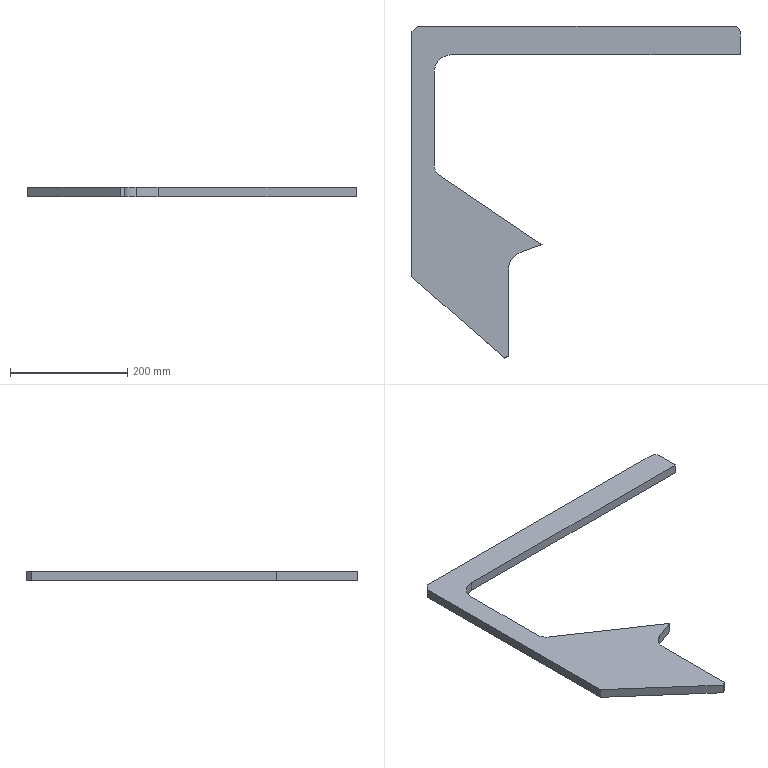Part | SolidWorks | features Extrusion 1 | 1 solid | 17 faces | box 560 x 566.399 x 16 mm | volume 1167723 mm3 | plane 13 | cylinder 4 | commonest cylinder face diameters 60 x2 20 x1 40 x1
STEP:
#1=CARTESIAN_POINT('',(560.,563.,0.));
#2=VERTEX_POINT('',#1);
#3=CARTESIAN_POINT('',(550.,573.,0.));
#4=VERTEX_POINT('',#3);
#5=CARTESIAN_POINT('',(550.,563.,0.));
#6=DIRECTION('',(0.,0.,1.));
#7=DIRECTION('',(1.,0.,0.));
#8=AXIS2_PLACEMENT_3D('',#5,#6,#7);
#9=CIRCLE('',#8,10.);
#10=EDGE_CURVE('',#2,#4,#9,.T.);
#11=ORIENTED_EDGE('',*,*,#10,.T.);
#12=CARTESIAN_POINT('',(550.,573.,16.));
#13=VERTEX_POINT('',#12);
#14=CARTESIAN_POINT('',(550.,573.,16.));
#15=DIRECTION('',(0.,0.,-1.));
#16=VECTOR('',#15,1000.);
#17=LINE('',#14,#16);
#18=EDGE_CURVE('',#13,#4,#17,.T.);
#19=ORIENTED_EDGE('',*,*,#18,.F.);
#20=CARTESIAN_POINT('',(560.,563.,16.));
#21=VERTEX_POINT('',#20);
#22=CARTESIAN_POINT('',(550.,563.,16.));
#23=DIRECTION('',(0.,0.,1.));
#24=DIRECTION('',(1.,0.,0.));
#25=AXIS2_PLACEMENT_3D('',#22,#23,#24);
#26=CIRCLE('',#25,10.);
#27=EDGE_CURVE('',#21,#13,#26,.T.);
#28=ORIENTED_EDGE('',*,*,#27,.F.);
#29=CARTESIAN_POINT('',(560.,563.,16.));
#30=DIRECTION('',(0.,0.,-1.));
#31=VECTOR('',#30,1000.);
#32=LINE('',#29,#31);
#33=EDGE_CURVE('',#21,#2,#32,.T.);
#34=ORIENTED_EDGE('',*,*,#33,.T.);
#35=EDGE_LOOP('',(#11,#19,#28,#34));
#36=FACE_OUTER_BOUND('',#35,.T.);
#37=CARTESIAN_POINT('',(550.,563.,16.));
#38=DIRECTION('',(0.,0.,-1.));
#39=DIRECTION('',(-1.,0.,0.));
#40=AXIS2_PLACEMENT_3D('',#37,#38,#39);
#41=CYLINDRICAL_SURFACE('',#40,10.);
#42=ADVANCED_FACE('',(#36),#41,.T.);
#43=CARTESIAN_POINT('',(10.,573.,0.));
#44=VERTEX_POINT('',#43);
#45=CARTESIAN_POINT('',(10.,573.,0.));
#46=DIRECTION('',(-1.,0.,0.));
#47=VECTOR('',#46,1000.);
#48=LINE('',#45,#47);
#49=EDGE_CURVE('',#4,#44,#48,.T.);
#50=ORIENTED_EDGE('',*,*,#49,.T.);
#51=CARTESIAN_POINT('',(10.,573.,16.));
#52=VERTEX_POINT('',#51);
#53=CARTESIAN_POINT('',(10.,573.,16.));
#54=DIRECTION('',(0.,0.,-1.));
#55=VECTOR('',#54,1000.);
#56=LINE('',#53,#55);
#57=EDGE_CURVE('',#52,#44,#56,.T.);
#58=ORIENTED_EDGE('',*,*,#57,.F.);
#59=CARTESIAN_POINT('',(10.,573.,16.));
#60=DIRECTION('',(-1.,0.,0.));
#61=VECTOR('',#60,1000.);
#62=LINE('',#59,#61);
#63=EDGE_CURVE('',#13,#52,#62,.T.);
#64=ORIENTED_EDGE('',*,*,#63,.F.);
#65=ORIENTED_EDGE('',*,*,#18,.T.);
#66=EDGE_LOOP('',(#50,#58,#64,#65));
#67=FACE_OUTER_BOUND('',#66,.T.);
#68=CARTESIAN_POINT('',(10.,573.,16.));
#69=DIRECTION('',(0.,-1.,0.));
#70=DIRECTION('',(0.,0.,-1.));
#71=AXIS2_PLACEMENT_3D('',#68,#69,#70);
#72=PLANE('',#71);
#73=ADVANCED_FACE('',(#67),#72,.F.);
#74=CARTESIAN_POINT('',(0.,563.,0.));
#75=VERTEX_POINT('',#74);
#76=CARTESIAN_POINT('',(0.,563.,0.));
#77=DIRECTION('',(-0.7071,-0.7071,0.));
#78=VECTOR('',#77,1000.);
#79=LINE('',#76,#78);
#80=EDGE_CURVE('',#44,#75,#79,.T.);
#81=ORIENTED_EDGE('',*,*,#80,.T.);
#82=CARTESIAN_POINT('',(0.,563.,16.));
#83=VERTEX_POINT('',#82);
#84=CARTESIAN_POINT('',(0.,563.,16.));
#85=DIRECTION('',(0.,0.,-1.));
#86=VECTOR('',#85,1000.);
#87=LINE('',#84,#86);
#88=EDGE_CURVE('',#83,#75,#87,.T.);
#89=ORIENTED_EDGE('',*,*,#88,.F.);
#90=CARTESIAN_POINT('',(0.,563.,16.));
#91=DIRECTION('',(-0.7071,-0.7071,0.));
#92=VECTOR('',#91,1000.);
#93=LINE('',#90,#92);
#94=EDGE_CURVE('',#52,#83,#93,.T.);
#95=ORIENTED_EDGE('',*,*,#94,.F.);
#96=ORIENTED_EDGE('',*,*,#57,.T.);
#97=EDGE_LOOP('',(#81,#89,#95,#96));
#98=FACE_OUTER_BOUND('',#97,.T.);
#99=CARTESIAN_POINT('',(0.,563.,16.));
#100=DIRECTION('',(0.7071,-0.7071,0.));
#101=DIRECTION('',(0.7071,0.7071,0.));
#102=AXIS2_PLACEMENT_3D('',#99,#100,#101);
#103=PLANE('',#102);
#104=ADVANCED_FACE('',(#98),#103,.F.);
#105=CARTESIAN_POINT('',(0.,145.,0.));
#106=VERTEX_POINT('',#105);
#107=CARTESIAN_POINT('',(0.,145.,0.));
#108=DIRECTION('',(0.,-1.,0.));
#109=VECTOR('',#108,1000.);
#110=LINE('',#107,#109);
#111=EDGE_CURVE('',#75,#106,#110,.T.);
#112=ORIENTED_EDGE('',*,*,#111,.T.);
#113=CARTESIAN_POINT('',(0.,145.,16.));
#114=VERTEX_POINT('',#113);
#115=CARTESIAN_POINT('',(0.,145.,16.));
#116=DIRECTION('',(0.,0.,-1.));
#117=VECTOR('',#116,1000.);
#118=LINE('',#115,#117);
#119=EDGE_CURVE('',#114,#106,#118,.T.);
#120=ORIENTED_EDGE('',*,*,#119,.F.);
#121=CARTESIAN_POINT('',(0.,145.,16.));
#122=DIRECTION('',(0.,-1.,0.));
#123=VECTOR('',#122,1000.);
#124=LINE('',#121,#123);
#125=EDGE_CURVE('',#83,#114,#124,.T.);
#126=ORIENTED_EDGE('',*,*,#125,.F.);
#127=ORIENTED_EDGE('',*,*,#88,.T.);
#128=EDGE_LOOP('',(#112,#120,#126,#127));
#129=FACE_OUTER_BOUND('',#128,.T.);
#130=CARTESIAN_POINT('',(0.,145.,16.));
#131=DIRECTION('',(1.,0.,0.));
#132=DIRECTION('',(0.,0.,-1.));
#133=AXIS2_PLACEMENT_3D('',#130,#131,#132);
#134=PLANE('',#133);
#135=ADVANCED_FACE('',(#129),#134,.F.);
#136=CARTESIAN_POINT('',(157.488,6.601,0.));
#137=VERTEX_POINT('',#136);
#138=CARTESIAN_POINT('',(157.488,6.601,0.));
#139=DIRECTION('',(0.7512,-0.6601,0.));
#140=VECTOR('',#139,1000.);
#141=LINE('',#138,#140);
#142=EDGE_CURVE('',#106,#137,#141,.T.);
#143=ORIENTED_EDGE('',*,*,#142,.T.);
#144=CARTESIAN_POINT('',(157.488,6.601,16.));
#145=VERTEX_POINT('',#144);
#146=CARTESIAN_POINT('',(157.488,6.601,16.));
#147=DIRECTION('',(0.,0.,-1.));
#148=VECTOR('',#147,1000.);
#149=LINE('',#146,#148);
#150=EDGE_CURVE('',#145,#137,#149,.T.);
#151=ORIENTED_EDGE('',*,*,#150,.F.);
#152=CARTESIAN_POINT('',(157.488,6.601,16.));
#153=DIRECTION('',(0.7512,-0.6601,0.));
#154=VECTOR('',#153,1000.);
#155=LINE('',#152,#154);
#156=EDGE_CURVE('',#114,#145,#155,.T.);
#157=ORIENTED_EDGE('',*,*,#156,.F.);
#158=ORIENTED_EDGE('',*,*,#119,.T.);
#159=EDGE_LOOP('',(#143,#151,#157,#158));
#160=FACE_OUTER_BOUND('',#159,.T.);
#161=CARTESIAN_POINT('',(157.488,6.601,16.));
#162=DIRECTION('',(0.6601,0.7512,0.));
#163=DIRECTION('',(-0.7512,0.6601,0.));
#164=AXIS2_PLACEMENT_3D('',#161,#162,#163);
#165=PLANE('',#164);
#166=ADVANCED_FACE('',(#160),#165,.F.);
#167=CARTESIAN_POINT('',(165.,10.,0.));
#168=VERTEX_POINT('',#167);
#169=CARTESIAN_POINT('',(165.,10.,0.));
#170=DIRECTION('',(0.9111,0.4122,0.));
#171=VECTOR('',#170,1000.);
#172=LINE('',#169,#171);
#173=EDGE_CURVE('',#137,#168,#172,.T.);
#174=ORIENTED_EDGE('',*,*,#173,.T.);
#175=CARTESIAN_POINT('',(165.,10.,16.));
#176=VERTEX_POINT('',#175);
#177=CARTESIAN_POINT('',(165.,10.,16.));
#178=DIRECTION('',(0.,0.,-1.));
#179=VECTOR('',#178,1000.);
#180=LINE('',#177,#179);
#181=EDGE_CURVE('',#176,#168,#180,.T.);
#182=ORIENTED_EDGE('',*,*,#181,.F.);
#183=CARTESIAN_POINT('',(165.,10.,16.));
#184=DIRECTION('',(0.9111,0.4122,0.));
#185=VECTOR('',#184,1000.);
#186=LINE('',#183,#185);
#187=EDGE_CURVE('',#145,#176,#186,.T.);
#188=ORIENTED_EDGE('',*,*,#187,.F.);
#189=ORIENTED_EDGE('',*,*,#150,.T.);
#190=EDGE_LOOP('',(#174,#182,#188,#189));
#191=FACE_OUTER_BOUND('',#190,.T.);
#192=CARTESIAN_POINT('',(165.,10.,16.));
#193=DIRECTION('',(-0.4122,0.9111,0.));
#194=DIRECTION('',(-0.9111,-0.4122,0.));
#195=AXIS2_PLACEMENT_3D('',#192,#193,#194);
#196=PLANE('',#195);
#197=ADVANCED_FACE('',(#191),#196,.F.);
#198=CARTESIAN_POINT('',(165.,158.408,0.));
#199=VERTEX_POINT('',#198);
#200=CARTESIAN_POINT('',(165.,158.408,0.));
#201=DIRECTION('',(0.,1.,0.));
#202=VECTOR('',#201,1000.);
#203=LINE('',#200,#202);
#204=EDGE_CURVE('',#168,#199,#203,.T.);
#205=ORIENTED_EDGE('',*,*,#204,.T.);
#206=CARTESIAN_POINT('',(165.,158.408,16.));
#207=VERTEX_POINT('',#206);
#208=CARTESIAN_POINT('',(165.,158.408,16.));
#209=DIRECTION('',(0.,0.,-1.));
#210=VECTOR('',#209,1000.);
#211=LINE('',#208,#210);
#212=EDGE_CURVE('',#207,#199,#211,.T.);
#213=ORIENTED_EDGE('',*,*,#212,.F.);
#214=CARTESIAN_POINT('',(165.,158.408,16.));
#215=DIRECTION('',(0.,1.,0.));
#216=VECTOR('',#215,1000.);
#217=LINE('',#214,#216);
#218=EDGE_CURVE('',#176,#207,#217,.T.);
#219=ORIENTED_EDGE('',*,*,#218,.F.);
#220=ORIENTED_EDGE('',*,*,#181,.T.);
#221=EDGE_LOOP('',(#205,#213,#219,#220));
#222=FACE_OUTER_BOUND('',#221,.T.);
#223=CARTESIAN_POINT('',(165.,158.408,16.));
#224=DIRECTION('',(-1.,0.,0.));
#225=DIRECTION('',(0.,-1.,0.));
#226=AXIS2_PLACEMENT_3D('',#223,#224,#225);
#227=PLANE('',#226);
#228=ADVANCED_FACE('',(#222),#227,.F.);
#229=CARTESIAN_POINT('',(184.847,186.638,0.));
#230=VERTEX_POINT('',#229);
#231=CARTESIAN_POINT('',(195.,158.408,0.));
#232=DIRECTION('',(0.,0.,-1.));
#233=DIRECTION('',(1.,0.,0.));
#234=AXIS2_PLACEMENT_3D('',#231,#232,#233);
#235=CIRCLE('',#234,30.);
#236=EDGE_CURVE('',#199,#230,#235,.T.);
#237=ORIENTED_EDGE('',*,*,#236,.T.);
#238=CARTESIAN_POINT('',(184.847,186.638,16.));
#239=VERTEX_POINT('',#238);
#240=CARTESIAN_POINT('',(184.847,186.638,16.));
#241=DIRECTION('',(0.,0.,-1.));
#242=VECTOR('',#241,1000.);
#243=LINE('',#240,#242);
#244=EDGE_CURVE('',#239,#230,#243,.T.);
#245=ORIENTED_EDGE('',*,*,#244,.F.);
#246=CARTESIAN_POINT('',(195.,158.408,16.));
#247=DIRECTION('',(0.,0.,-1.));
#248=DIRECTION('',(1.,0.,0.));
#249=AXIS2_PLACEMENT_3D('',#246,#247,#248);
#250=CIRCLE('',#249,30.);
#251=EDGE_CURVE('',#207,#239,#250,.T.);
#252=ORIENTED_EDGE('',*,*,#251,.F.);
#253=ORIENTED_EDGE('',*,*,#212,.T.);
#254=EDGE_LOOP('',(#237,#245,#252,#253));
#255=FACE_OUTER_BOUND('',#254,.T.);
#256=CARTESIAN_POINT('',(195.,158.408,16.));
#257=DIRECTION('',(0.,0.,-1.));
#258=DIRECTION('',(-1.,0.,0.));
#259=AXIS2_PLACEMENT_3D('',#256,#257,#258);
#260=CYLINDRICAL_SURFACE('',#259,30.);
#261=ADVANCED_FACE('',(#255),#260,.F.);
#262=CARTESIAN_POINT('',(222.,200.,0.));
#263=VERTEX_POINT('',#262);
#264=CARTESIAN_POINT('',(222.,200.,0.));
#265=DIRECTION('',(0.941,0.3384,0.));
#266=VECTOR('',#265,1000.);
#267=LINE('',#264,#266);
#268=EDGE_CURVE('',#230,#263,#267,.T.);
#269=ORIENTED_EDGE('',*,*,#268,.T.);
#270=CARTESIAN_POINT('',(222.,200.,16.));
#271=VERTEX_POINT('',#270);
#272=CARTESIAN_POINT('',(222.,200.,16.));
#273=DIRECTION('',(0.,0.,-1.));
#274=VECTOR('',#273,1000.);
#275=LINE('',#272,#274);
#276=EDGE_CURVE('',#271,#263,#275,.T.);
#277=ORIENTED_EDGE('',*,*,#276,.F.);
#278=CARTESIAN_POINT('',(222.,200.,16.));
#279=DIRECTION('',(0.941,0.3384,0.));
#280=VECTOR('',#279,1000.);
#281=LINE('',#278,#280);
#282=EDGE_CURVE('',#239,#271,#281,.T.);
#283=ORIENTED_EDGE('',*,*,#282,.F.);
#284=ORIENTED_EDGE('',*,*,#244,.T.);
#285=EDGE_LOOP('',(#269,#277,#283,#284));
#286=FACE_OUTER_BOUND('',#285,.T.);
#287=CARTESIAN_POINT('',(222.,200.,16.));
#288=DIRECTION('',(-0.3384,0.941,0.));
#289=DIRECTION('',(-0.941,-0.3384,0.));
#290=AXIS2_PLACEMENT_3D('',#287,#288,#289);
#291=PLANE('',#290);
#292=ADVANCED_FACE('',(#286),#291,.F.);
#293=CARTESIAN_POINT('',(46.811,318.253,0.));
#294=VERTEX_POINT('',#293);
#295=CARTESIAN_POINT('',(46.811,318.253,0.));
#296=DIRECTION('',(-0.8288,0.5595,0.));
#297=VECTOR('',#296,1000.);
#298=LINE('',#295,#297);
#299=EDGE_CURVE('',#263,#294,#298,.T.);
#300=ORIENTED_EDGE('',*,*,#299,.T.);
#301=CARTESIAN_POINT('',(46.811,318.253,16.));
#302=VERTEX_POINT('',#301);
#303=CARTESIAN_POINT('',(46.811,318.253,16.));
#304=DIRECTION('',(0.,0.,-1.));
#305=VECTOR('',#304,1000.);
#306=LINE('',#303,#305);
#307=EDGE_CURVE('',#302,#294,#306,.T.);
#308=ORIENTED_EDGE('',*,*,#307,.F.);
#309=CARTESIAN_POINT('',(46.811,318.253,16.));
#310=DIRECTION('',(-0.8288,0.5595,0.));
#311=VECTOR('',#310,1000.);
#312=LINE('',#309,#311);
#313=EDGE_CURVE('',#271,#302,#312,.T.);
#314=ORIENTED_EDGE('',*,*,#313,.F.);
#315=ORIENTED_EDGE('',*,*,#276,.T.);
#316=EDGE_LOOP('',(#300,#308,#314,#315));
#317=FACE_OUTER_BOUND('',#316,.T.);
#318=CARTESIAN_POINT('',(46.811,318.253,16.));
#319=DIRECTION('',(-0.5595,-0.8288,0.));
#320=DIRECTION('',(0.8288,-0.5595,0.));
#321=AXIS2_PLACEMENT_3D('',#318,#319,#320);
#322=PLANE('',#321);
#323=ADVANCED_FACE('',(#317),#322,.F.);
#324=CARTESIAN_POINT('',(38.,334.83,0.));
#325=VERTEX_POINT('',#324);
#326=CARTESIAN_POINT('',(58.,334.83,0.));
#327=DIRECTION('',(0.,0.,-1.));
#328=DIRECTION('',(1.,0.,0.));
#329=AXIS2_PLACEMENT_3D('',#326,#327,#328);
#330=CIRCLE('',#329,20.);
#331=EDGE_CURVE('',#294,#325,#330,.T.);
#332=ORIENTED_EDGE('',*,*,#331,.T.);
#333=CARTESIAN_POINT('',(38.,334.83,16.));
#334=VERTEX_POINT('',#333);
#335=CARTESIAN_POINT('',(38.,334.83,16.));
#336=DIRECTION('',(0.,0.,-1.));
#337=VECTOR('',#336,1000.);
#338=LINE('',#335,#337);
#339=EDGE_CURVE('',#334,#325,#338,.T.);
#340=ORIENTED_EDGE('',*,*,#339,.F.);
#341=CARTESIAN_POINT('',(58.,334.83,16.));
#342=DIRECTION('',(0.,0.,-1.));
#343=DIRECTION('',(1.,0.,0.));
#344=AXIS2_PLACEMENT_3D('',#341,#342,#343);
#345=CIRCLE('',#344,20.);
#346=EDGE_CURVE('',#302,#334,#345,.T.);
#347=ORIENTED_EDGE('',*,*,#346,.F.);
#348=ORIENTED_EDGE('',*,*,#307,.T.);
#349=EDGE_LOOP('',(#332,#340,#347,#348));
#350=FACE_OUTER_BOUND('',#349,.T.);
#351=CARTESIAN_POINT('',(58.,334.83,16.));
#352=DIRECTION('',(0.,0.,-1.));
#353=DIRECTION('',(-1.,0.,0.));
#354=AXIS2_PLACEMENT_3D('',#351,#352,#353);
#355=CYLINDRICAL_SURFACE('',#354,20.);
#356=ADVANCED_FACE('',(#350),#355,.F.);
#357=CARTESIAN_POINT('',(38.,494.,0.));
#358=VERTEX_POINT('',#357);
#359=CARTESIAN_POINT('',(38.,494.,0.));
#360=DIRECTION('',(0.,1.,0.));
#361=VECTOR('',#360,1000.);
#362=LINE('',#359,#361);
#363=EDGE_CURVE('',#325,#358,#362,.T.);
#364=ORIENTED_EDGE('',*,*,#363,.T.);
#365=CARTESIAN_POINT('',(38.,494.,16.));
#366=VERTEX_POINT('',#365);
#367=CARTESIAN_POINT('',(38.,494.,16.));
#368=DIRECTION('',(0.,0.,-1.));
#369=VECTOR('',#368,1000.);
#370=LINE('',#367,#369);
#371=EDGE_CURVE('',#366,#358,#370,.T.);
#372=ORIENTED_EDGE('',*,*,#371,.F.);
#373=CARTESIAN_POINT('',(38.,494.,16.));
#374=DIRECTION('',(0.,1.,0.));
#375=VECTOR('',#374,1000.);
#376=LINE('',#373,#375);
#377=EDGE_CURVE('',#334,#366,#376,.T.);
#378=ORIENTED_EDGE('',*,*,#377,.F.);
#379=ORIENTED_EDGE('',*,*,#339,.T.);
#380=EDGE_LOOP('',(#364,#372,#378,#379));
#381=FACE_OUTER_BOUND('',#380,.T.);
#382=CARTESIAN_POINT('',(38.,494.,16.));
#383=DIRECTION('',(-1.,0.,0.));
#384=DIRECTION('',(0.,-1.,0.));
#385=AXIS2_PLACEMENT_3D('',#382,#383,#384);
#386=PLANE('',#385);
#387=ADVANCED_FACE('',(#381),#386,.F.);
#388=CARTESIAN_POINT('',(68.,524.,0.));
#389=VERTEX_POINT('',#388);
#390=CARTESIAN_POINT('',(68.,494.,0.));
#391=DIRECTION('',(0.,0.,-1.));
#392=DIRECTION('',(1.,0.,0.));
#393=AXIS2_PLACEMENT_3D('',#390,#391,#392);
#394=CIRCLE('',#393,30.);
#395=EDGE_CURVE('',#358,#389,#394,.T.);
#396=ORIENTED_EDGE('',*,*,#395,.T.);
#397=CARTESIAN_POINT('',(68.,524.,16.));
#398=VERTEX_POINT('',#397);
#399=CARTESIAN_POINT('',(68.,524.,16.));
#400=DIRECTION('',(0.,0.,-1.));
#401=VECTOR('',#400,1000.);
#402=LINE('',#399,#401);
#403=EDGE_CURVE('',#398,#389,#402,.T.);
#404=ORIENTED_EDGE('',*,*,#403,.F.);
#405=CARTESIAN_POINT('',(68.,494.,16.));
#406=DIRECTION('',(0.,0.,-1.));
#407=DIRECTION('',(1.,0.,0.));
#408=AXIS2_PLACEMENT_3D('',#405,#406,#407);
#409=CIRCLE('',#408,30.);
#410=EDGE_CURVE('',#366,#398,#409,.T.);
#411=ORIENTED_EDGE('',*,*,#410,.F.);
#412=ORIENTED_EDGE('',*,*,#371,.T.);
#413=EDGE_LOOP('',(#396,#404,#411,#412));
#414=FACE_OUTER_BOUND('',#413,.T.);
#415=CARTESIAN_POINT('',(68.,494.,16.));
#416=DIRECTION('',(0.,0.,-1.));
#417=DIRECTION('',(-1.,0.,0.));
#418=AXIS2_PLACEMENT_3D('',#415,#416,#417);
#419=CYLINDRICAL_SURFACE('',#418,30.);
#420=ADVANCED_FACE('',(#414),#419,.F.);
#421=CARTESIAN_POINT('',(560.,524.,0.));
#422=VERTEX_POINT('',#421);
#423=CARTESIAN_POINT('',(560.,524.,0.));
#424=DIRECTION('',(1.,0.,0.));
#425=VECTOR('',#424,1000.);
#426=LINE('',#423,#425);
#427=EDGE_CURVE('',#389,#422,#426,.T.);
#428=ORIENTED_EDGE('',*,*,#427,.T.);
#429=CARTESIAN_POINT('',(560.,524.,16.));
#430=VERTEX_POINT('',#429);
#431=CARTESIAN_POINT('',(560.,524.,16.));
#432=DIRECTION('',(0.,0.,-1.));
#433=VECTOR('',#432,1000.);
#434=LINE('',#431,#433);
#435=EDGE_CURVE('',#430,#422,#434,.T.);
#436=ORIENTED_EDGE('',*,*,#435,.F.);
#437=CARTESIAN_POINT('',(560.,524.,16.));
#438=DIRECTION('',(1.,0.,0.));
#439=VECTOR('',#438,1000.);
#440=LINE('',#437,#439);
#441=EDGE_CURVE('',#398,#430,#440,.T.);
#442=ORIENTED_EDGE('',*,*,#441,.F.);
#443=ORIENTED_EDGE('',*,*,#403,.T.);
#444=EDGE_LOOP('',(#428,#436,#442,#443));
#445=FACE_OUTER_BOUND('',#444,.T.);
#446=CARTESIAN_POINT('',(560.,524.,16.));
#447=DIRECTION('',(0.,1.,0.));
#448=DIRECTION('',(-1.,0.,0.));
#449=AXIS2_PLACEMENT_3D('',#446,#447,#448);
#450=PLANE('',#449);
#451=ADVANCED_FACE('',(#445),#450,.F.);
#452=CARTESIAN_POINT('',(560.,563.,0.));
#453=DIRECTION('',(0.,1.,0.));
#454=VECTOR('',#453,1000.);
#455=LINE('',#452,#454);
#456=EDGE_CURVE('',#422,#2,#455,.T.);
#457=ORIENTED_EDGE('',*,*,#456,.T.);
#458=ORIENTED_EDGE('',*,*,#33,.F.);
#459=CARTESIAN_POINT('',(560.,563.,16.));
#460=DIRECTION('',(0.,1.,0.));
#461=VECTOR('',#460,1000.);
#462=LINE('',#459,#461);
#463=EDGE_CURVE('',#430,#21,#462,.T.);
#464=ORIENTED_EDGE('',*,*,#463,.F.);
#465=ORIENTED_EDGE('',*,*,#435,.T.);
#466=EDGE_LOOP('',(#457,#458,#464,#465));
#467=FACE_OUTER_BOUND('',#466,.T.);
#468=CARTESIAN_POINT('',(560.,563.,16.));
#469=DIRECTION('',(-1.,0.,0.));
#470=DIRECTION('',(0.,0.,1.));
#471=AXIS2_PLACEMENT_3D('',#468,#469,#470);
#472=PLANE('',#471);
#473=ADVANCED_FACE('',(#467),#472,.F.);
#474=ORIENTED_EDGE('',*,*,#27,.T.);
#475=ORIENTED_EDGE('',*,*,#63,.T.);
#476=ORIENTED_EDGE('',*,*,#94,.T.);
#477=ORIENTED_EDGE('',*,*,#125,.T.);
#478=ORIENTED_EDGE('',*,*,#156,.T.);
#479=ORIENTED_EDGE('',*,*,#187,.T.);
#480=ORIENTED_EDGE('',*,*,#218,.T.);
#481=ORIENTED_EDGE('',*,*,#251,.T.);
#482=ORIENTED_EDGE('',*,*,#282,.T.);
#483=ORIENTED_EDGE('',*,*,#313,.T.);
#484=ORIENTED_EDGE('',*,*,#346,.T.);
#485=ORIENTED_EDGE('',*,*,#377,.T.);
#486=ORIENTED_EDGE('',*,*,#410,.T.);
#487=ORIENTED_EDGE('',*,*,#441,.T.);
#488=ORIENTED_EDGE('',*,*,#463,.T.);
#489=EDGE_LOOP('',(#474,#475,#476,#477,#478,#479,#480,#481,#482,#483,#484,#485,#486,#487,#488));
#490=FACE_OUTER_BOUND('',#489,.T.);
#491=CARTESIAN_POINT('',(550.,563.,16.));
#492=DIRECTION('',(0.,0.,1.));
#493=DIRECTION('',(1.,0.,0.));
#494=AXIS2_PLACEMENT_3D('',#491,#492,#493);
#495=PLANE('',#494);
#496=ADVANCED_FACE('',(#490),#495,.T.);
#497=ORIENTED_EDGE('',*,*,#10,.F.);
#498=ORIENTED_EDGE('',*,*,#456,.F.);
#499=ORIENTED_EDGE('',*,*,#427,.F.);
#500=ORIENTED_EDGE('',*,*,#395,.F.);
#501=ORIENTED_EDGE('',*,*,#363,.F.);
#502=ORIENTED_EDGE('',*,*,#331,.F.);
#503=ORIENTED_EDGE('',*,*,#299,.F.);
#504=ORIENTED_EDGE('',*,*,#268,.F.);
#505=ORIENTED_EDGE('',*,*,#236,.F.);
#506=ORIENTED_EDGE('',*,*,#204,.F.);
#507=ORIENTED_EDGE('',*,*,#173,.F.);
#508=ORIENTED_EDGE('',*,*,#142,.F.);
#509=ORIENTED_EDGE('',*,*,#111,.F.);
#510=ORIENTED_EDGE('',*,*,#80,.F.);
#511=ORIENTED_EDGE('',*,*,#49,.F.);
#512=EDGE_LOOP('',(#497,#498,#499,#500,#501,#502,#503,#504,#505,#506,#507,#508,#509,#510,#511));
#513=FACE_OUTER_BOUND('',#512,.T.);
#514=CARTESIAN_POINT('',(550.,563.,0.));
#515=DIRECTION('',(0.,0.,1.));
#516=DIRECTION('',(1.,0.,0.));
#517=AXIS2_PLACEMENT_3D('',#514,#515,#516);
#518=PLANE('',#517);
#519=ADVANCED_FACE('',(#513),#518,.F.);
#520=CLOSED_SHELL('',(#42,#73,#104,#135,#166,#197,#228,#261,#292,#323,#356,#387,#420,#451,#473,#496,#519));
#521=MANIFOLD_SOLID_BREP('',#520);
#522=CARTESIAN_POINT('',(0.,0.,0.));
#523=DIRECTION('',(0.,0.,1.));
#524=DIRECTION('',(1.,0.,0.));
#525=AXIS2_PLACEMENT_3D('',#522,#523,#524);
#526=(LENGTH_UNIT()NAMED_UNIT(*)SI_UNIT(.MILLI.,.METRE.));
#527=UNCERTAINTY_MEASURE_WITH_UNIT(LENGTH_MEASURE(0.00001),#526,'','');
#528=(NAMED_UNIT(*)PLANE_ANGLE_UNIT()SI_UNIT($,.RADIAN.));
#529=(NAMED_UNIT(*)SI_UNIT($,.STERADIAN.)SOLID_ANGLE_UNIT());
#530=(GEOMETRIC_REPRESENTATION_CONTEXT(3)GLOBAL_UNCERTAINTY_ASSIGNED_CONTEXT((#527))GLOBAL_UNIT_ASSIGNED_CONTEXT((#526,#528,#529))REPRESENTATION_CONTEXT('',''));
#531=ADVANCED_BREP_SHAPE_REPRESENTATION('',(#521,#525),#530);